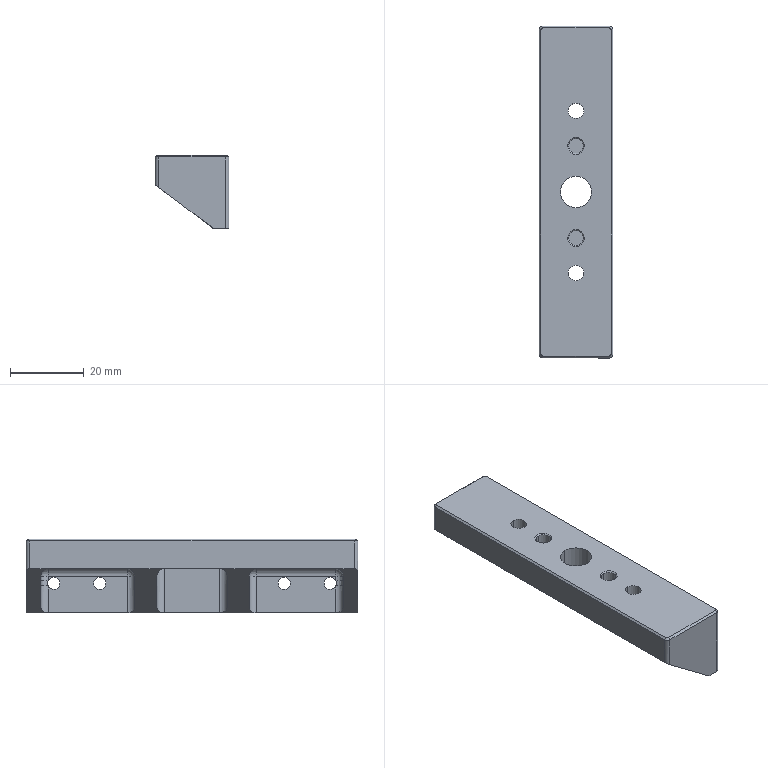NC program | NX | posted with a generic post | part box 20 x 90 x 20 mm
Lines 15909 to 15930 of 15930:
(PLANAR_MILL_COPY_COPY_COPY_COPY_1 , TOOL : D6A45)
N31804 T01 M6
N31806 G54
N31808 G17 G0 G90 X-47.1 Y4.73 B0. C0. S9500 M3
N31810 G43 Z30. H1
N31812 Z0.5
N31814 G94 G1 Z-1. F1250.
N31816 X-46.4 Y5.134
N31818 G3 X-45.9 Y6. R1.
N31820 G1 Y9.
N31822 G2 X-44. Y10.9 R1.9
N31824 G1 X44.
N31826 G2 X45.9 Y9. R1.9
N31828 G1 Y6.
N31830 G3 X46.4 Y5.134 R1.
N31832 G1 X47.1 Y4.73
N31834 Z0.5
N31836 G0 Z30.
N31838 M5
N31840 M2